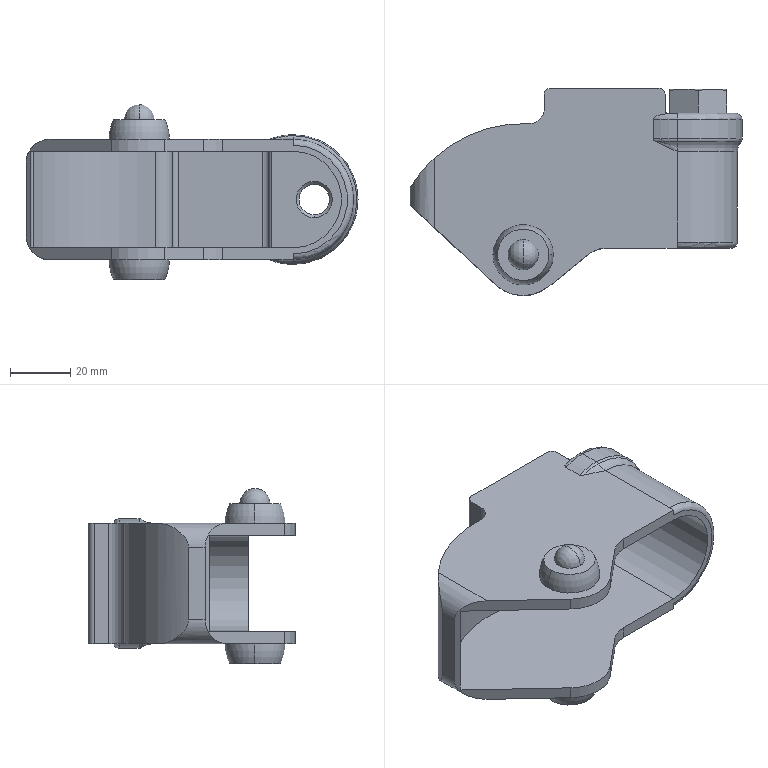Part | SolidWorks | features BaseBody 1 | 1 solid | 93 faces | box 110 x 68.7 x 58 mm | volume 68662 mm3 | plane 38 | cylinder 28 | torus 14 | cone 11 | sphere 2 | commonest cylinder face diameters 4 x5 43 x3 2 x2 8.4 x2 10 x2 10.106 x2